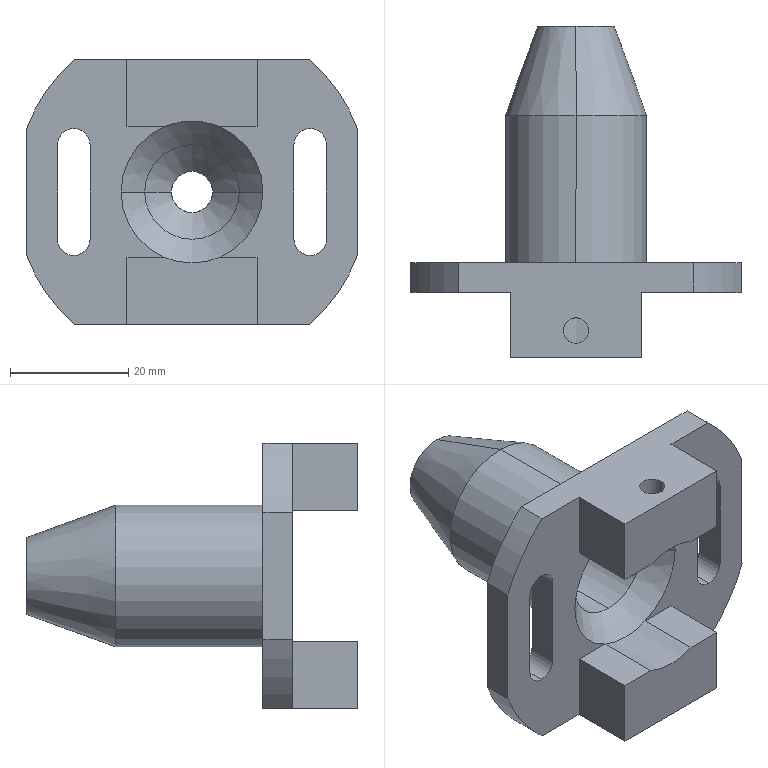Part | SolidWorks | features BaseBody 1 | 1 solid | 49 faces | box 56 x 56 x 45 mm | volume 24024 mm3 | plane 22 | cylinder 21 | cone 6 | commonest cylinder face diameters 5.5 x6 24 x5 60 x4 4.3 x2 7 x2 16 x2